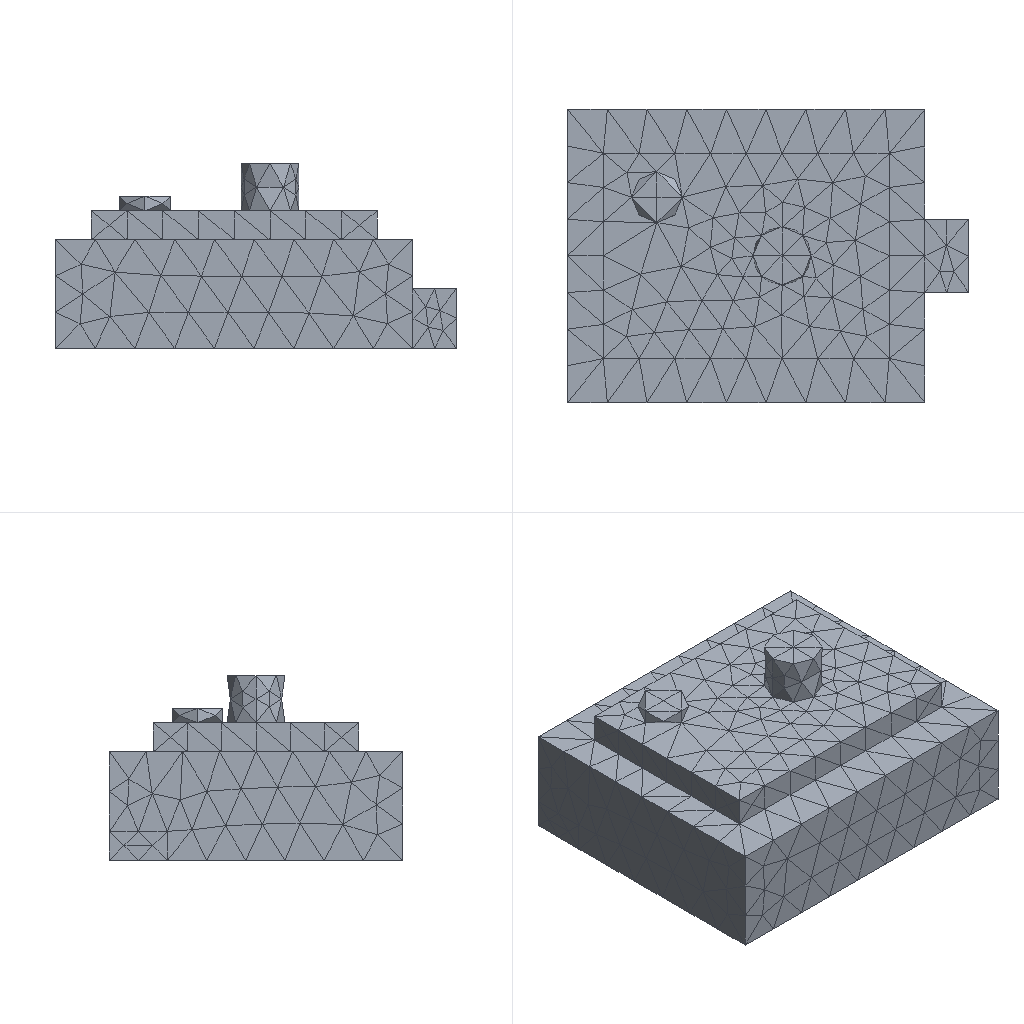Simulation study | ansys mapdl
Set-up summary:
category,name,step,type,value,unit,region
solver,ansys_mapdl
units,mm-N-s-tonne (MPa),,inferred,E=210000 density=
analysis,model,,static
mesh,nodes,,,4532
mesh,elements,,,2727
element_type,SOLID187,,,2727
material,mat 1,,E,210000
material,mat 1,,nu,0.3
load,,model,body load temp,,,all
load,,model,force,"1000 [dir=(0, 0, -1) n=153]",,node list
bc,,model,fixed,"[dofs=UX,UY,UZ n=4508]",,node list
Ansys APDL input file, long lists of numbers shortened:
/COM,ANSYS RELEASE 2026 R1           BUILD 26.1      UP20260202       09:11:26
/PREP7
/NOPR
/TITLE,2
ANTYPE, 0
*IF,_CDRDOFF,EQ,1,THEN     !if solid model was read in
_CDRDOFF=             !reset flag, numoffs already performed
*ELSE              !offset database for the following FE model
NUMOFF,NODE,     4532
NUMOFF,ELEM,     2727
NUMOFF,MAT ,        1
NUMOFF,TYPE,        1
*ENDIF
*SET,_RETURN ,  0.
*SET,_STATUS ,  0.
*SET,_UIQR   ,  153.
*SET,__FLOATPARAMETER__,  4532.
DOF,DELETE
ETBLOCK,        1,        1
(2i9,19a9)
        1      187        0        0        0        0        0        0        0        0        0        0        0        0        0        0        0        0        0        0        0
       -1
NBLOCK,6,SOLID,      4532,      4532
(3i9,6e21.13e3)
        1        0        0-3.3375000000000E+001 4.0500000000000E+001 8.0000000000000E+000
! (4531 more lines like these left out)
N,UNBL,LOC,       -1,
EBLOCK,19,SOLID,      2727,      2727
(19i10)
         1         1         1         1         0         0         0         0        10         0         1      1707      1708      1709      1710      1969      1970      1971      1972
! (5453 more lines like these left out)
        -1
MPTEMP,UNBL, 1, 1,  0.    ,
MPDATA,UNBL, 1,EX  ,       1, 1,  210000.000    ,
MPTEMP,UNBL, 1, 1,  0.    ,
MPDATA,UNBL, 1,NUXY,       1, 1, 0.3    ,
MPTEMP,UNBL, 1, 1,  0.    ,
MPDATA,UNBL, 1,PRXY,       1, 1, 0.3    ,
EXTOPT,ATTR,      0,      0,      0
EXTOPT,ESIZE,  0,  0.
EXTOPT,ACLEAR,      0
TREF,  0.
IRLF,  0
BFUNIF,TEMP,_TINY
ACEL,  0.    ,  0.    ,  0.
OMEGA,  0.    ,  0.    ,  0.
DOMEGA,  0.    ,  0.    ,  0.
CGLOC,  0.    ,  0.    ,  0.
CGOMEGA,  0.    ,  0.    ,  0.
DCGOMG,  0.    ,  0.    ,  0.
KUSE,     0
TIME,  0.
ALPHAD,  0.
BETAD,  0.
DMPRAT,  0.
DMPSTR,  0.
CRPLIM, 0.1    ,   0
CRPLIM,  0.    ,   1
NCNV,     0, 1.000000000E+12,     0,  0.    ,  0.
NEQIT,     0
ERESX,DEFA
DBLOCK,      4508
(i9,a6,2(pg16.9))
        1  UX    0.00000000      0.00000000
! (4507 more lines like these left out)
       -1
FBLOCK,       153
(i9,a6,2(pg16.9))
      829  FZ   -6.53594771      0.00000000
! (152 more lines like these left out)
       -1
/GO
FINISH
Results summary:
result,analysis_type_db,,,static,unstated
result,n_sets,,,1,unstated
result,load_steps[0].set,load_step=1,,1,unstated
result,load_steps[0].substep,load_step=1,,1,unstated
result,load_steps[0].time,load_step=1,,1,unstated
result,load_steps[0].freq,load_step=1,,1,unstated
result,load_steps[0].max_usum,load_step=1,,0.0004349,unstated
result,load_steps[0].max_seqv,load_step=1,,5.711,unstated
result,load_steps[0].reaction_sum.FX,load_step=1,,-6.33704e-12,unstated
result,load_steps[0].reaction_sum.FY,load_step=1,,1.82223e-11,unstated
result,load_steps[0].reaction_sum.FZ,load_step=1,,1000,unstated
result,load_steps[0].reaction_sum.MX,load_step=1,,0,unstated
result,load_steps[0].reaction_sum.MY,load_step=1,,0,unstated
result,load_steps[0].reaction_sum.MZ,load_step=1,,0,unstated
result,convergence,,,results present for all listed sets,unstated